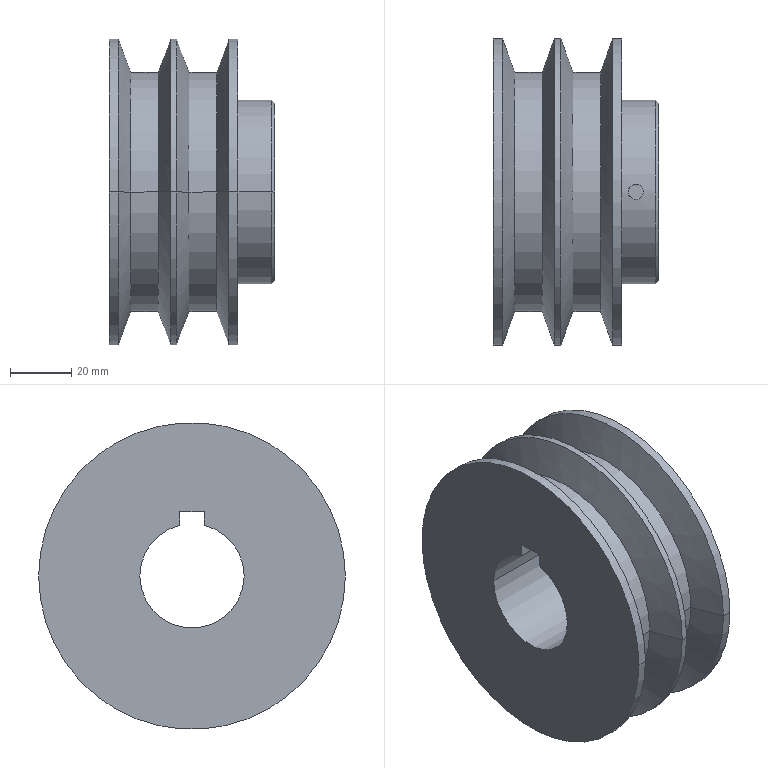Part | SolidWorks | features ICE 2, Chamfer 1, HoleWzd 1, Revolution 1 | 1 solid | 33 faces | box 54 x 100 x 100 mm | volume 231745 mm3 | cylinder 17 | cone 10 | plane 6 | commonest cylinder face diameters 100 x6 78 x4 34 x3 5 x2 60 x2
STEP:
#1=CARTESIAN_POINT('',(54.,29.,0.));
#2=VERTEX_POINT('',#1);
#3=CARTESIAN_POINT('',(54.,-29.,0.));
#4=VERTEX_POINT('',#3);
#5=CARTESIAN_POINT('',(54.,0.,0.));
#6=DIRECTION('',(1.,0.,0.));
#7=DIRECTION('',(0.,1.,0.));
#8=AXIS2_PLACEMENT_3D('',#5,#6,#7);
#9=CIRCLE('',#8,29.);
#10=EDGE_CURVE('',#2,#4,#9,.T.);
#11=ORIENTED_EDGE('',*,*,#10,.F.);
#12=CARTESIAN_POINT('',(53.,30.,0.));
#13=VERTEX_POINT('',#12);
#14=CARTESIAN_POINT('',(54.,29.,0.));
#15=DIRECTION('',(-0.7071,0.7071,0.));
#16=VECTOR('',#15,1000.);
#17=LINE('',#14,#16);
#18=EDGE_CURVE('',#2,#13,#17,.T.);
#19=ORIENTED_EDGE('',*,*,#18,.T.);
#20=CARTESIAN_POINT('',(53.,-30.,0.));
#21=VERTEX_POINT('',#20);
#22=CARTESIAN_POINT('',(53.,0.,0.));
#23=DIRECTION('',(-1.,0.,0.));
#24=DIRECTION('',(0.,1.,0.));
#25=AXIS2_PLACEMENT_3D('',#22,#23,#24);
#26=CIRCLE('',#25,30.);
#27=EDGE_CURVE('',#21,#13,#26,.T.);
#28=ORIENTED_EDGE('',*,*,#27,.F.);
#29=CARTESIAN_POINT('',(54.,-29.,0.));
#30=DIRECTION('',(-0.7071,-0.7071,0.));
#31=VECTOR('',#30,1000.);
#32=LINE('',#29,#31);
#33=EDGE_CURVE('',#4,#21,#32,.T.);
#34=ORIENTED_EDGE('',*,*,#33,.F.);
#35=EDGE_LOOP('',(#11,#19,#28,#34));
#36=FACE_OUTER_BOUND('',#35,.T.);
#37=CARTESIAN_POINT('',(54.,0.,0.));
#38=DIRECTION('',(-1.,0.,0.));
#39=DIRECTION('',(0.,-1.,0.));
#40=AXIS2_PLACEMENT_3D('',#37,#38,#39);
#41=CONICAL_SURFACE('',#40,29.,0.7854);
#42=ADVANCED_FACE('',(#36),#41,.T.);
#43=CARTESIAN_POINT('',(44.,0.,30.));
#44=VERTEX_POINT('',#43);
#45=CARTESIAN_POINT('',(49.,0.,30.));
#46=VERTEX_POINT('',#45);
#47=CARTESIAN_POINT('',(44.,0.,30.));
#48=CARTESIAN_POINT('',(44.,-0.1653,30.));
#49=CARTESIAN_POINT('',(44.016,-0.3277,29.999));
#50=CARTESIAN_POINT('',(44.08,-0.6474,29.993));
#51=CARTESIAN_POINT('',(44.128,-0.8062,29.99));
#52=CARTESIAN_POINT('',(44.253,-1.109,29.98));
#53=CARTESIAN_POINT('',(44.33,-1.253,29.974));
#54=CARTESIAN_POINT('',(44.512,-1.524,29.962));
#55=CARTESIAN_POINT('',(44.617,-1.653,29.955));
#56=CARTESIAN_POINT('',(44.848,-1.883,29.941));
#57=CARTESIAN_POINT('',(44.974,-1.987,29.934));
#58=CARTESIAN_POINT('',(45.247,-2.17,29.922));
#59=CARTESIAN_POINT('',(45.392,-2.247,29.916));
#60=CARTESIAN_POINT('',(45.693,-2.372,29.906));
#61=CARTESIAN_POINT('',(45.851,-2.42,29.902));
#62=CARTESIAN_POINT('',(46.174,-2.484,29.897));
#63=CARTESIAN_POINT('',(46.336,-2.5,29.896));
#64=CARTESIAN_POINT('',(46.662,-2.5,29.896));
#65=CARTESIAN_POINT('',(46.828,-2.484,29.897));
#66=CARTESIAN_POINT('',(47.149,-2.42,29.902));
#67=CARTESIAN_POINT('',(47.305,-2.373,29.906));
#68=CARTESIAN_POINT('',(47.607,-2.247,29.916));
#69=CARTESIAN_POINT('',(47.754,-2.169,29.922));
#70=CARTESIAN_POINT('',(48.024,-1.988,29.934));
#71=CARTESIAN_POINT('',(48.151,-1.885,29.941));
#72=CARTESIAN_POINT('',(48.384,-1.651,29.955));
#73=CARTESIAN_POINT('',(48.488,-1.525,29.962));
#74=CARTESIAN_POINT('',(48.669,-1.254,29.974));
#75=CARTESIAN_POINT('',(48.747,-1.108,29.98));
#76=CARTESIAN_POINT('',(48.872,-0.8053,29.99));
#77=CARTESIAN_POINT('',(48.92,-0.6495,29.993));
#78=CARTESIAN_POINT('',(48.984,-0.329,29.999));
#79=CARTESIAN_POINT('',(49.,-0.1632,30.));
#80=CARTESIAN_POINT('',(49.,0.,30.));
#81=B_SPLINE_CURVE_WITH_KNOTS('',3,(#47,#48,#49,#50,#51,#52,#53,#54,#55,#56,#57,#58,#59,#60,#61,#62,#63,#64,#65,#66,#67,#68,#69,#70,#71,#72,#73,#74,#75,#76,#77,#78,#79,#80),.UNSPECIFIED.,.F.,.F.,(4,2,2,2,2,2,2,2,2,2,2,2,2,2,2,2,4),(0.,0.0004887,0.0009774,0.001466,0.001955,0.002444,0.002932,0.003421,0.00391,0.004398,0.004887,0.005376,0.005865,0.006353,0.006842,0.007331,0.00782),.UNSPECIFIED.);
#82=EDGE_CURVE('',#44,#46,#81,.T.);
#83=ORIENTED_EDGE('',*,*,#82,.T.);
#84=CARTESIAN_POINT('',(49.,0.,21.));
#85=VERTEX_POINT('',#84);
#86=CARTESIAN_POINT('',(49.,0.,0.));
#87=DIRECTION('',(0.,0.,-1.));
#88=VECTOR('',#87,1000.);
#89=LINE('',#86,#88);
#90=EDGE_CURVE('',#46,#85,#89,.T.);
#91=ORIENTED_EDGE('',*,*,#90,.T.);
#92=CARTESIAN_POINT('',(44.,0.,21.));
#93=VERTEX_POINT('',#92);
#94=CARTESIAN_POINT('',(46.5,0.,21.));
#95=DIRECTION('',(0.,0.,-1.));
#96=DIRECTION('',(1.,0.,0.));
#97=AXIS2_PLACEMENT_3D('',#94,#95,#96);
#98=CIRCLE('',#97,2.5);
#99=EDGE_CURVE('',#85,#93,#98,.T.);
#100=ORIENTED_EDGE('',*,*,#99,.T.);
#101=CARTESIAN_POINT('',(44.,0.,0.));
#102=DIRECTION('',(0.,0.,-1.));
#103=VECTOR('',#102,1000.);
#104=LINE('',#101,#103);
#105=EDGE_CURVE('',#44,#93,#104,.T.);
#106=ORIENTED_EDGE('',*,*,#105,.F.);
#107=EDGE_LOOP('',(#83,#91,#100,#106));
#108=FACE_OUTER_BOUND('',#107,.T.);
#109=CARTESIAN_POINT('',(46.5,0.,0.));
#110=DIRECTION('',(0.,0.,-1.));
#111=DIRECTION('',(-1.,0.,0.));
#112=AXIS2_PLACEMENT_3D('',#109,#110,#111);
#113=CYLINDRICAL_SURFACE('',#112,2.5);
#114=ADVANCED_FACE('',(#108),#113,.F.);
#115=CARTESIAN_POINT('',(0.,17.,0.));
#116=VERTEX_POINT('',#115);
#117=CARTESIAN_POINT('',(0.,-17.,0.));
#118=VERTEX_POINT('',#117);
#119=CARTESIAN_POINT('',(0.,0.,0.));
#120=DIRECTION('',(-1.,0.,0.));
#121=DIRECTION('',(0.,-1.,0.));
#122=AXIS2_PLACEMENT_3D('',#119,#120,#121);
#123=CIRCLE('',#122,17.);
#124=EDGE_CURVE('',#116,#118,#123,.T.);
#125=ORIENTED_EDGE('',*,*,#124,.T.);
#126=CARTESIAN_POINT('',(54.,-17.,0.));
#127=VERTEX_POINT('',#126);
#128=CARTESIAN_POINT('',(-16.,-17.,0.));
#129=DIRECTION('',(1.,0.,0.));
#130=VECTOR('',#129,1000.);
#131=LINE('',#128,#130);
#132=EDGE_CURVE('',#118,#127,#131,.T.);
#133=ORIENTED_EDGE('',*,*,#132,.T.);
#134=CARTESIAN_POINT('',(54.,17.,0.));
#135=VERTEX_POINT('',#134);
#136=CARTESIAN_POINT('',(54.,0.,0.));
#137=DIRECTION('',(1.,0.,0.));
#138=DIRECTION('',(0.,1.,0.));
#139=AXIS2_PLACEMENT_3D('',#136,#137,#138);
#140=CIRCLE('',#139,17.);
#141=EDGE_CURVE('',#127,#135,#140,.T.);
#142=ORIENTED_EDGE('',*,*,#141,.T.);
#143=CARTESIAN_POINT('',(-16.,17.,0.));
#144=DIRECTION('',(1.,0.,0.));
#145=VECTOR('',#144,1000.);
#146=LINE('',#143,#145);
#147=EDGE_CURVE('',#116,#135,#146,.T.);
#148=ORIENTED_EDGE('',*,*,#147,.F.);
#149=EDGE_LOOP('',(#125,#133,#142,#148));
#150=FACE_OUTER_BOUND('',#149,.T.);
#151=CARTESIAN_POINT('',(-16.,0.,0.));
#152=DIRECTION('',(1.,0.,0.));
#153=DIRECTION('',(0.,1.,0.));
#154=AXIS2_PLACEMENT_3D('',#151,#152,#153);
#155=CYLINDRICAL_SURFACE('',#154,17.);
#156=ADVANCED_FACE('',(#150),#155,.F.);
#157=CARTESIAN_POINT('',(0.,4.,16.523));
#158=VERTEX_POINT('',#157);
#159=CARTESIAN_POINT('',(0.,0.,0.));
#160=DIRECTION('',(-1.,0.,0.));
#161=DIRECTION('',(0.,-1.,0.));
#162=AXIS2_PLACEMENT_3D('',#159,#160,#161);
#163=CIRCLE('',#162,17.);
#164=EDGE_CURVE('',#158,#116,#163,.T.);
#165=ORIENTED_EDGE('',*,*,#164,.T.);
#166=ORIENTED_EDGE('',*,*,#147,.T.);
#167=CARTESIAN_POINT('',(54.,4.,16.523));
#168=VERTEX_POINT('',#167);
#169=CARTESIAN_POINT('',(54.,0.,0.));
#170=DIRECTION('',(1.,0.,0.));
#171=DIRECTION('',(0.,1.,0.));
#172=AXIS2_PLACEMENT_3D('',#169,#170,#171);
#173=CIRCLE('',#172,17.);
#174=EDGE_CURVE('',#135,#168,#173,.T.);
#175=ORIENTED_EDGE('',*,*,#174,.T.);
#176=CARTESIAN_POINT('',(-16.,4.,16.523));
#177=DIRECTION('',(-1.,0.,0.));
#178=VECTOR('',#177,1000.);
#179=LINE('',#176,#178);
#180=EDGE_CURVE('',#168,#158,#179,.T.);
#181=ORIENTED_EDGE('',*,*,#180,.T.);
#182=EDGE_LOOP('',(#165,#166,#175,#181));
#183=FACE_OUTER_BOUND('',#182,.T.);
#184=CARTESIAN_POINT('',(-16.,0.,0.));
#185=DIRECTION('',(1.,0.,0.));
#186=DIRECTION('',(0.,1.,0.));
#187=AXIS2_PLACEMENT_3D('',#184,#185,#186);
#188=CYLINDRICAL_SURFACE('',#187,17.);
#189=ADVANCED_FACE('',(#183),#188,.F.);
#190=ORIENTED_EDGE('',*,*,#82,.F.);
#191=CARTESIAN_POINT('',(49.,0.,30.));
#192=CARTESIAN_POINT('',(49.,0.1632,30.));
#193=CARTESIAN_POINT('',(48.984,0.3254,29.999));
#194=CARTESIAN_POINT('',(48.92,0.6478,29.993));
#195=CARTESIAN_POINT('',(48.872,0.8057,29.99));
#196=CARTESIAN_POINT('',(48.748,1.107,29.98));
#197=CARTESIAN_POINT('',(48.67,1.252,29.974));
#198=CARTESIAN_POINT('',(48.488,1.525,29.962));
#199=CARTESIAN_POINT('',(48.384,1.651,29.955));
#200=CARTESIAN_POINT('',(48.154,1.882,29.941));
#201=CARTESIAN_POINT('',(48.025,1.987,29.934));
#202=CARTESIAN_POINT('',(47.754,2.169,29.922));
#203=CARTESIAN_POINT('',(47.61,2.246,29.916));
#204=CARTESIAN_POINT('',(47.308,2.372,29.906));
#205=CARTESIAN_POINT('',(47.149,2.42,29.902));
#206=CARTESIAN_POINT('',(46.829,2.484,29.897));
#207=CARTESIAN_POINT('',(46.667,2.5,29.896));
#208=CARTESIAN_POINT('',(46.337,2.5,29.896));
#209=CARTESIAN_POINT('',(46.174,2.484,29.897));
#210=CARTESIAN_POINT('',(45.854,2.421,29.902));
#211=CARTESIAN_POINT('',(45.696,2.373,29.906));
#212=CARTESIAN_POINT('',(45.393,2.247,29.916));
#213=CARTESIAN_POINT('',(45.249,2.171,29.921));
#214=CARTESIAN_POINT('',(44.978,1.99,29.934));
#215=CARTESIAN_POINT('',(44.849,1.884,29.941));
#216=CARTESIAN_POINT('',(44.618,1.654,29.955));
#217=CARTESIAN_POINT('',(44.515,1.528,29.961));
#218=CARTESIAN_POINT('',(44.332,1.255,29.974));
#219=CARTESIAN_POINT('',(44.254,1.11,29.98));
#220=CARTESIAN_POINT('',(44.066,0.6587,29.994));
#221=CARTESIAN_POINT('',(44.,0.3304,30.));
#222=CARTESIAN_POINT('',(44.,0.,30.));
#223=B_SPLINE_CURVE_WITH_KNOTS('',3,(#191,#192,#193,#194,#195,#196,#197,#198,#199,#200,#201,#202,#203,#204,#205,#206,#207,#208,#209,#210,#211,#212,#213,#214,#215,#216,#217,#218,#219,#220,#221,#222),.UNSPECIFIED.,.F.,.F.,(4,2,2,2,2,2,2,2,2,2,2,2,2,2,2,4),(0.00782,0.008308,0.008797,0.009285,0.009774,0.01026,0.01075,0.01124,0.01173,0.01222,0.01271,0.01319,0.01368,0.01417,0.01466,0.01564),.UNSPECIFIED.);
#224=EDGE_CURVE('',#46,#44,#223,.T.);
#225=ORIENTED_EDGE('',*,*,#224,.F.);
#226=EDGE_LOOP('',(#190,#225));
#227=FACE_BOUND('',#226,.T.);
#228=CARTESIAN_POINT('',(42.,30.,0.));
#229=VERTEX_POINT('',#228);
#230=CARTESIAN_POINT('',(42.,-30.,0.));
#231=VERTEX_POINT('',#230);
#232=CARTESIAN_POINT('',(42.,0.,0.));
#233=DIRECTION('',(1.,0.,0.));
#234=DIRECTION('',(0.,1.,0.));
#235=AXIS2_PLACEMENT_3D('',#232,#233,#234);
#236=CIRCLE('',#235,30.);
#237=EDGE_CURVE('',#229,#231,#236,.T.);
#238=ORIENTED_EDGE('',*,*,#237,.T.);
#239=CARTESIAN_POINT('',(54.,-30.,0.));
#240=DIRECTION('',(1.,0.,0.));
#241=VECTOR('',#240,1000.);
#242=LINE('',#239,#241);
#243=EDGE_CURVE('',#231,#21,#242,.T.);
#244=ORIENTED_EDGE('',*,*,#243,.T.);
#245=ORIENTED_EDGE('',*,*,#27,.T.);
#246=CARTESIAN_POINT('',(54.,30.,0.));
#247=DIRECTION('',(1.,0.,0.));
#248=VECTOR('',#247,1000.);
#249=LINE('',#246,#248);
#250=EDGE_CURVE('',#229,#13,#249,.T.);
#251=ORIENTED_EDGE('',*,*,#250,.F.);
#252=EDGE_LOOP('',(#238,#244,#245,#251));
#253=FACE_OUTER_BOUND('',#252,.T.);
#254=CARTESIAN_POINT('',(54.,0.,0.));
#255=DIRECTION('',(1.,0.,0.));
#256=DIRECTION('',(0.,1.,0.));
#257=AXIS2_PLACEMENT_3D('',#254,#255,#256);
#258=CYLINDRICAL_SURFACE('',#257,30.);
#259=ADVANCED_FACE('',(#227,#253),#258,.T.);
#260=CARTESIAN_POINT('',(39.,50.,0.));
#261=VERTEX_POINT('',#260);
#262=CARTESIAN_POINT('',(39.,-50.,0.));
#263=VERTEX_POINT('',#262);
#264=CARTESIAN_POINT('',(39.,0.,0.));
#265=DIRECTION('',(1.,0.,0.));
#266=DIRECTION('',(0.,1.,0.));
#267=AXIS2_PLACEMENT_3D('',#264,#265,#266);
#268=CIRCLE('',#267,50.);
#269=EDGE_CURVE('',#261,#263,#268,.T.);
#270=ORIENTED_EDGE('',*,*,#269,.T.);
#271=CARTESIAN_POINT('',(42.,-50.,0.));
#272=VERTEX_POINT('',#271);
#273=CARTESIAN_POINT('',(54.,-50.,0.));
#274=DIRECTION('',(1.,0.,0.));
#275=VECTOR('',#274,1000.);
#276=LINE('',#273,#275);
#277=EDGE_CURVE('',#263,#272,#276,.T.);
#278=ORIENTED_EDGE('',*,*,#277,.T.);
#279=CARTESIAN_POINT('',(42.,50.,0.));
#280=VERTEX_POINT('',#279);
#281=CARTESIAN_POINT('',(42.,0.,0.));
#282=DIRECTION('',(1.,0.,0.));
#283=DIRECTION('',(0.,1.,0.));
#284=AXIS2_PLACEMENT_3D('',#281,#282,#283);
#285=CIRCLE('',#284,50.);
#286=EDGE_CURVE('',#280,#272,#285,.T.);
#287=ORIENTED_EDGE('',*,*,#286,.F.);
#288=CARTESIAN_POINT('',(54.,50.,0.));
#289=DIRECTION('',(1.,0.,0.));
#290=VECTOR('',#289,1000.);
#291=LINE('',#288,#290);
#292=EDGE_CURVE('',#261,#280,#291,.T.);
#293=ORIENTED_EDGE('',*,*,#292,.F.);
#294=EDGE_LOOP('',(#270,#278,#287,#293));
#295=FACE_OUTER_BOUND('',#294,.T.);
#296=CARTESIAN_POINT('',(54.,0.,0.));
#297=DIRECTION('',(1.,0.,0.));
#298=DIRECTION('',(0.,1.,0.));
#299=AXIS2_PLACEMENT_3D('',#296,#297,#298);
#300=CYLINDRICAL_SURFACE('',#299,50.);
#301=ADVANCED_FACE('',(#295),#300,.T.);
#302=CARTESIAN_POINT('',(34.996,39.,0.));
#303=VERTEX_POINT('',#302);
#304=CARTESIAN_POINT('',(34.996,-39.,0.));
#305=VERTEX_POINT('',#304);
#306=CARTESIAN_POINT('',(34.996,0.,0.));
#307=DIRECTION('',(1.,0.,0.));
#308=DIRECTION('',(0.,1.,0.));
#309=AXIS2_PLACEMENT_3D('',#306,#307,#308);
#310=CIRCLE('',#309,39.);
#311=EDGE_CURVE('',#303,#305,#310,.T.);
#312=ORIENTED_EDGE('',*,*,#311,.T.);
#313=CARTESIAN_POINT('',(39.,-50.,0.));
#314=DIRECTION('',(0.342,-0.9397,0.));
#315=VECTOR('',#314,1000.);
#316=LINE('',#313,#315);
#317=EDGE_CURVE('',#305,#263,#316,.T.);
#318=ORIENTED_EDGE('',*,*,#317,.T.);
#319=ORIENTED_EDGE('',*,*,#269,.F.);
#320=CARTESIAN_POINT('',(39.,50.,0.));
#321=DIRECTION('',(0.342,0.9397,0.));
#322=VECTOR('',#321,1000.);
#323=LINE('',#320,#322);
#324=EDGE_CURVE('',#303,#261,#323,.T.);
#325=ORIENTED_EDGE('',*,*,#324,.F.);
#326=EDGE_LOOP('',(#312,#318,#319,#325));
#327=FACE_OUTER_BOUND('',#326,.T.);
#328=CARTESIAN_POINT('',(39.,0.,0.));
#329=DIRECTION('',(1.,0.,0.));
#330=DIRECTION('',(0.,1.,0.));
#331=AXIS2_PLACEMENT_3D('',#328,#329,#330);
#332=CONICAL_SURFACE('',#331,50.,1.222);
#333=ADVANCED_FACE('',(#327),#332,.T.);
#334=CARTESIAN_POINT('',(26.004,39.,0.));
#335=VERTEX_POINT('',#334);
#336=CARTESIAN_POINT('',(26.004,-39.,0.));
#337=VERTEX_POINT('',#336);
#338=CARTESIAN_POINT('',(26.004,0.,0.));
#339=DIRECTION('',(1.,0.,0.));
#340=DIRECTION('',(0.,1.,0.));
#341=AXIS2_PLACEMENT_3D('',#338,#339,#340);
#342=CIRCLE('',#341,39.);
#343=EDGE_CURVE('',#335,#337,#342,.T.);
#344=ORIENTED_EDGE('',*,*,#343,.T.);
#345=CARTESIAN_POINT('',(54.,-39.,0.));
#346=DIRECTION('',(1.,0.,0.));
#347=VECTOR('',#346,1000.);
#348=LINE('',#345,#347);
#349=EDGE_CURVE('',#337,#305,#348,.T.);
#350=ORIENTED_EDGE('',*,*,#349,.T.);
#351=ORIENTED_EDGE('',*,*,#311,.F.);
#352=CARTESIAN_POINT('',(54.,39.,0.));
#353=DIRECTION('',(1.,0.,0.));
#354=VECTOR('',#353,1000.);
#355=LINE('',#352,#354);
#356=EDGE_CURVE('',#335,#303,#355,.T.);
#357=ORIENTED_EDGE('',*,*,#356,.F.);
#358=EDGE_LOOP('',(#344,#350,#351,#357));
#359=FACE_OUTER_BOUND('',#358,.T.);
#360=CARTESIAN_POINT('',(54.,0.,0.));
#361=DIRECTION('',(1.,0.,0.));
#362=DIRECTION('',(0.,1.,0.));
#363=AXIS2_PLACEMENT_3D('',#360,#361,#362);
#364=CYLINDRICAL_SURFACE('',#363,39.);
#365=ADVANCED_FACE('',(#359),#364,.T.);
#366=ORIENTED_EDGE('',*,*,#343,.F.);
#367=CARTESIAN_POINT('',(22.,50.,0.));
#368=VERTEX_POINT('',#367);
#369=CARTESIAN_POINT('',(26.004,39.,0.));
#370=DIRECTION('',(-0.342,0.9397,0.));
#371=VECTOR('',#370,1000.);
#372=LINE('',#369,#371);
#373=EDGE_CURVE('',#335,#368,#372,.T.);
#374=ORIENTED_EDGE('',*,*,#373,.T.);
#375=CARTESIAN_POINT('',(22.,-50.,0.));
#376=VERTEX_POINT('',#375);
#377=CARTESIAN_POINT('',(22.,0.,0.));
#378=DIRECTION('',(1.,0.,0.));
#379=DIRECTION('',(0.,1.,0.));
#380=AXIS2_PLACEMENT_3D('',#377,#378,#379);
#381=CIRCLE('',#380,50.);
#382=EDGE_CURVE('',#368,#376,#381,.T.);
#383=ORIENTED_EDGE('',*,*,#382,.T.);
#384=CARTESIAN_POINT('',(26.004,-39.,0.));
#385=DIRECTION('',(-0.342,-0.9397,0.));
#386=VECTOR('',#385,1000.);
#387=LINE('',#384,#386);
#388=EDGE_CURVE('',#337,#376,#387,.T.);
#389=ORIENTED_EDGE('',*,*,#388,.F.);
#390=EDGE_LOOP('',(#366,#374,#383,#389));
#391=FACE_OUTER_BOUND('',#390,.T.);
#392=CARTESIAN_POINT('',(26.004,0.,0.));
#393=DIRECTION('',(-1.,0.,0.));
#394=DIRECTION('',(0.,-1.,0.));
#395=AXIS2_PLACEMENT_3D('',#392,#393,#394);
#396=CONICAL_SURFACE('',#395,39.,1.222);
#397=ADVANCED_FACE('',(#391),#396,.T.);
#398=CARTESIAN_POINT('',(20.,50.,0.));
#399=VERTEX_POINT('',#398);
#400=CARTESIAN_POINT('',(20.,-50.,0.));
#401=VERTEX_POINT('',#400);
#402=CARTESIAN_POINT('',(20.,0.,0.));
#403=DIRECTION('',(1.,0.,0.));
#404=DIRECTION('',(0.,1.,0.));
#405=AXIS2_PLACEMENT_3D('',#402,#403,#404);
#406=CIRCLE('',#405,50.);
#407=EDGE_CURVE('',#399,#401,#406,.T.);
#408=ORIENTED_EDGE('',*,*,#407,.T.);
#409=CARTESIAN_POINT('',(54.,-50.,0.));
#410=DIRECTION('',(1.,0.,0.));
#411=VECTOR('',#410,1000.);
#412=LINE('',#409,#411);
#413=EDGE_CURVE('',#401,#376,#412,.T.);
#414=ORIENTED_EDGE('',*,*,#413,.T.);
#415=ORIENTED_EDGE('',*,*,#382,.F.);
#416=CARTESIAN_POINT('',(54.,50.,0.));
#417=DIRECTION('',(1.,0.,0.));
#418=VECTOR('',#417,1000.);
#419=LINE('',#416,#418);
#420=EDGE_CURVE('',#399,#368,#419,.T.);
#421=ORIENTED_EDGE('',*,*,#420,.F.);
#422=EDGE_LOOP('',(#408,#414,#415,#421));
#423=FACE_OUTER_BOUND('',#422,.T.);
#424=CARTESIAN_POINT('',(54.,0.,0.));
#425=DIRECTION('',(1.,0.,0.));
#426=DIRECTION('',(0.,1.,0.));
#427=AXIS2_PLACEMENT_3D('',#424,#425,#426);
#428=CYLINDRICAL_SURFACE('',#427,50.);
#429=ADVANCED_FACE('',(#423),#428,.T.);
#430=CARTESIAN_POINT('',(15.996,39.,0.));
#431=VERTEX_POINT('',#430);
#432=CARTESIAN_POINT('',(15.996,-39.,0.));
#433=VERTEX_POINT('',#432);
#434=CARTESIAN_POINT('',(15.996,0.,0.));
#435=DIRECTION('',(1.,0.,0.));
#436=DIRECTION('',(0.,1.,0.));
#437=AXIS2_PLACEMENT_3D('',#434,#435,#436);
#438=CIRCLE('',#437,39.);
#439=EDGE_CURVE('',#431,#433,#438,.T.);
#440=ORIENTED_EDGE('',*,*,#439,.T.);
#441=CARTESIAN_POINT('',(20.,-50.,0.));
#442=DIRECTION('',(0.342,-0.9397,0.));
#443=VECTOR('',#442,1000.);
#444=LINE('',#441,#443);
#445=EDGE_CURVE('',#433,#401,#444,.T.);
#446=ORIENTED_EDGE('',*,*,#445,.T.);
#447=ORIENTED_EDGE('',*,*,#407,.F.);
#448=CARTESIAN_POINT('',(20.,50.,0.));
#449=DIRECTION('',(0.342,0.9397,0.));
#450=VECTOR('',#449,1000.);
#451=LINE('',#448,#450);
#452=EDGE_CURVE('',#431,#399,#451,.T.);
#453=ORIENTED_EDGE('',*,*,#452,.F.);
#454=EDGE_LOOP('',(#440,#446,#447,#453));
#455=FACE_OUTER_BOUND('',#454,.T.);
#456=CARTESIAN_POINT('',(20.,0.,0.));
#457=DIRECTION('',(1.,0.,0.));
#458=DIRECTION('',(0.,1.,0.));
#459=AXIS2_PLACEMENT_3D('',#456,#457,#458);
#460=CONICAL_SURFACE('',#459,50.,1.222);
#461=ADVANCED_FACE('',(#455),#460,.T.);
#462=CARTESIAN_POINT('',(7.004,39.,0.));
#463=VERTEX_POINT('',#462);
#464=CARTESIAN_POINT('',(7.004,-39.,0.));
#465=VERTEX_POINT('',#464);
#466=CARTESIAN_POINT('',(7.004,0.,0.));
#467=DIRECTION('',(1.,0.,0.));
#468=DIRECTION('',(0.,1.,0.));
#469=AXIS2_PLACEMENT_3D('',#466,#467,#468);
#470=CIRCLE('',#469,39.);
#471=EDGE_CURVE('',#463,#465,#470,.T.);
#472=ORIENTED_EDGE('',*,*,#471,.T.);
#473=CARTESIAN_POINT('',(54.,-39.,0.));
#474=DIRECTION('',(1.,0.,0.));
#475=VECTOR('',#474,1000.);
#476=LINE('',#473,#475);
#477=EDGE_CURVE('',#465,#433,#476,.T.);
#478=ORIENTED_EDGE('',*,*,#477,.T.);
#479=ORIENTED_EDGE('',*,*,#439,.F.);
#480=CARTESIAN_POINT('',(54.,39.,0.));
#481=DIRECTION('',(1.,0.,0.));
#482=VECTOR('',#481,1000.);
#483=LINE('',#480,#482);
#484=EDGE_CURVE('',#463,#431,#483,.T.);
#485=ORIENTED_EDGE('',*,*,#484,.F.);
#486=EDGE_LOOP('',(#472,#478,#479,#485));
#487=FACE_OUTER_BOUND('',#486,.T.);
#488=CARTESIAN_POINT('',(54.,0.,0.));
#489=DIRECTION('',(1.,0.,0.));
#490=DIRECTION('',(0.,1.,0.));
#491=AXIS2_PLACEMENT_3D('',#488,#489,#490);
#492=CYLINDRICAL_SURFACE('',#491,39.);
#493=ADVANCED_FACE('',(#487),#492,.T.);
#494=ORIENTED_EDGE('',*,*,#471,.F.);
#495=CARTESIAN_POINT('',(3.,50.,0.));
#496=VERTEX_POINT('',#495);
#497=CARTESIAN_POINT('',(7.004,39.,0.));
#498=DIRECTION('',(-0.342,0.9397,0.));
#499=VECTOR('',#498,1000.);
#500=LINE('',#497,#499);
#501=EDGE_CURVE('',#463,#496,#500,.T.);
#502=ORIENTED_EDGE('',*,*,#501,.T.);
#503=CARTESIAN_POINT('',(3.,-50.,0.));
#504=VERTEX_POINT('',#503);
#505=CARTESIAN_POINT('',(3.,0.,0.));
#506=DIRECTION('',(1.,0.,0.));
#507=DIRECTION('',(0.,1.,0.));
#508=AXIS2_PLACEMENT_3D('',#505,#506,#507);
#509=CIRCLE('',#508,50.);
#510=EDGE_CURVE('',#496,#504,#509,.T.);
#511=ORIENTED_EDGE('',*,*,#510,.T.);
#512=CARTESIAN_POINT('',(7.004,-39.,0.));
#513=DIRECTION('',(-0.342,-0.9397,0.));
#514=VECTOR('',#513,1000.);
#515=LINE('',#512,#514);
#516=EDGE_CURVE('',#465,#504,#515,.T.);
#517=ORIENTED_EDGE('',*,*,#516,.F.);
#518=EDGE_LOOP('',(#494,#502,#511,#517));
#519=FACE_OUTER_BOUND('',#518,.T.);
#520=CARTESIAN_POINT('',(7.004,0.,0.));
#521=DIRECTION('',(-1.,0.,0.));
#522=DIRECTION('',(0.,-1.,0.));
#523=AXIS2_PLACEMENT_3D('',#520,#521,#522);
#524=CONICAL_SURFACE('',#523,39.,1.222);
#525=ADVANCED_FACE('',(#519),#524,.T.);
#526=CARTESIAN_POINT('',(0.,50.,0.));
#527=VERTEX_POINT('',#526);
#528=CARTESIAN_POINT('',(0.,-50.,0.));
#529=VERTEX_POINT('',#528);
#530=CARTESIAN_POINT('',(0.,0.,0.));
#531=DIRECTION('',(1.,0.,0.));
#532=DIRECTION('',(0.,1.,0.));
#533=AXIS2_PLACEMENT_3D('',#530,#531,#532);
#534=CIRCLE('',#533,50.);
#535=EDGE_CURVE('',#527,#529,#534,.T.);
#536=ORIENTED_EDGE('',*,*,#535,.T.);
#537=CARTESIAN_POINT('',(54.,-50.,0.));
#538=DIRECTION('',(1.,0.,0.));
#539=VECTOR('',#538,1000.);
#540=LINE('',#537,#539);
#541=EDGE_CURVE('',#529,#504,#540,.T.);
#542=ORIENTED_EDGE('',*,*,#541,.T.);
#543=ORIENTED_EDGE('',*,*,#510,.F.);
#544=CARTESIAN_POINT('',(54.,50.,0.));
#545=DIRECTION('',(1.,0.,0.));
#546=VECTOR('',#545,1000.);
#547=LINE('',#544,#546);
#548=EDGE_CURVE('',#527,#496,#547,.T.);
#549=ORIENTED_EDGE('',*,*,#548,.F.);
#550=EDGE_LOOP('',(#536,#542,#543,#549));
#551=FACE_OUTER_BOUND('',#550,.T.);
#552=CARTESIAN_POINT('',(54.,0.,0.));
#553=DIRECTION('',(1.,0.,0.));
#554=DIRECTION('',(0.,1.,0.));
#555=AXIS2_PLACEMENT_3D('',#552,#553,#554);
#556=CYLINDRICAL_SURFACE('',#555,50.);
#557=ADVANCED_FACE('',(#551),#556,.T.);
#558=CARTESIAN_POINT('',(0.,-4.,16.523));
#559=VERTEX_POINT('',#558);
#560=CARTESIAN_POINT('',(0.,-4.,21.));
#561=VERTEX_POINT('',#560);
#562=CARTESIAN_POINT('',(0.,-4.,0.));
#563=DIRECTION('',(0.,0.,1.));
#564=VECTOR('',#563,1000.);
#565=LINE('',#562,#564);
#566=EDGE_CURVE('',#559,#561,#565,.T.);
#567=ORIENTED_EDGE('',*,*,#566,.F.);
#568=CARTESIAN_POINT('',(0.,0.,0.));
#569=DIRECTION('',(-1.,0.,0.));
#570=DIRECTION('',(0.,-1.,0.));
#571=AXIS2_PLACEMENT_3D('',#568,#569,#570);
#572=CIRCLE('',#571,17.);
#573=EDGE_CURVE('',#118,#559,#572,.T.);
#574=ORIENTED_EDGE('',*,*,#573,.F.);
#575=ORIENTED_EDGE('',*,*,#124,.F.);
#576=ORIENTED_EDGE('',*,*,#164,.F.);
#577=CARTESIAN_POINT('',(0.,4.,21.));
#578=VERTEX_POINT('',#577);
#579=CARTESIAN_POINT('',(0.,4.,0.));
#580=DIRECTION('',(0.,0.,-1.));
#581=VECTOR('',#580,1000.);
#582=LINE('',#579,#581);
#583=EDGE_CURVE('',#578,#158,#582,.T.);
#584=ORIENTED_EDGE('',*,*,#583,.F.);
#585=CARTESIAN_POINT('',(0.,0.,21.));
#586=DIRECTION('',(0.,1.,0.));
#587=VECTOR('',#586,1000.);
#588=LINE('',#585,#587);
#589=EDGE_CURVE('',#561,#578,#588,.T.);
#590=ORIENTED_EDGE('',*,*,#589,.F.);
#591=EDGE_LOOP('',(#567,#574,#575,#576,#584,#590));
#592=FACE_BOUND('',#591,.T.);
#593=ORIENTED_EDGE('',*,*,#535,.F.);
#594=CARTESIAN_POINT('',(0.,0.,0.));
#595=DIRECTION('',(1.,0.,0.));
#596=DIRECTION('',(0.,1.,0.));
#597=AXIS2_PLACEMENT_3D('',#594,#595,#596);
#598=CIRCLE('',#597,50.);
#599=EDGE_CURVE('',#529,#527,#598,.T.);
#600=ORIENTED_EDGE('',*,*,#599,.F.);
#601=EDGE_LOOP('',(#593,#600));
#602=FACE_OUTER_BOUND('',#601,.T.);
#603=CARTESIAN_POINT('',(0.,0.,0.));
#604=DIRECTION('',(-1.,0.,0.));
#605=DIRECTION('',(0.,-1.,0.));
#606=AXIS2_PLACEMENT_3D('',#603,#604,#605);
#607=PLANE('',#606);
#608=ADVANCED_FACE('',(#592,#602),#607,.T.);
#609=ORIENTED_EDGE('',*,*,#541,.F.);
#610=ORIENTED_EDGE('',*,*,#599,.T.);
#611=ORIENTED_EDGE('',*,*,#548,.T.);
#612=CARTESIAN_POINT('',(3.,0.,0.));
#613=DIRECTION('',(1.,0.,0.));
#614=DIRECTION('',(0.,1.,0.));
#615=AXIS2_PLACEMENT_3D('',#612,#613,#614);
#616=CIRCLE('',#615,50.);
#617=EDGE_CURVE('',#504,#496,#616,.T.);
#618=ORIENTED_EDGE('',*,*,#617,.F.);
#619=EDGE_LOOP('',(#609,#610,#611,#618));
#620=FACE_OUTER_BOUND('',#619,.T.);
#621=CARTESIAN_POINT('',(54.,0.,0.));
#622=DIRECTION('',(1.,0.,0.));
#623=DIRECTION('',(0.,1.,0.));
#624=AXIS2_PLACEMENT_3D('',#621,#622,#623);
#625=CYLINDRICAL_SURFACE('',#624,50.);
#626=ADVANCED_FACE('',(#620),#625,.T.);
#627=ORIENTED_EDGE('',*,*,#501,.F.);
#628=CARTESIAN_POINT('',(7.004,0.,0.));
#629=DIRECTION('',(1.,0.,0.));
#630=DIRECTION('',(0.,1.,0.));
#631=AXIS2_PLACEMENT_3D('',#628,#629,#630);
#632=CIRCLE('',#631,39.);
#633=EDGE_CURVE('',#465,#463,#632,.T.);
#634=ORIENTED_EDGE('',*,*,#633,.F.);
#635=ORIENTED_EDGE('',*,*,#516,.T.);
#636=ORIENTED_EDGE('',*,*,#617,.T.);
#637=EDGE_LOOP('',(#627,#634,#635,#636));
#638=FACE_OUTER_BOUND('',#637,.T.);
#639=CARTESIAN_POINT('',(7.004,0.,0.));
#640=DIRECTION('',(-1.,0.,0.));
#641=DIRECTION('',(0.,-1.,0.));
#642=AXIS2_PLACEMENT_3D('',#639,#640,#641);
#643=CONICAL_SURFACE('',#642,39.,1.222);
#644=ADVANCED_FACE('',(#638),#643,.T.);
#645=ORIENTED_EDGE('',*,*,#477,.F.);
#646=ORIENTED_EDGE('',*,*,#633,.T.);
#647=ORIENTED_EDGE('',*,*,#484,.T.);
#648=CARTESIAN_POINT('',(15.996,0.,0.));
#649=DIRECTION('',(1.,0.,0.));
#650=DIRECTION('',(0.,1.,0.));
#651=AXIS2_PLACEMENT_3D('',#648,#649,#650);
#652=CIRCLE('',#651,39.);
#653=EDGE_CURVE('',#433,#431,#652,.T.);
#654=ORIENTED_EDGE('',*,*,#653,.F.);
#655=EDGE_LOOP('',(#645,#646,#647,#654));
#656=FACE_OUTER_BOUND('',#655,.T.);
#657=CARTESIAN_POINT('',(54.,0.,0.));
#658=DIRECTION('',(1.,0.,0.));
#659=DIRECTION('',(0.,1.,0.));
#660=AXIS2_PLACEMENT_3D('',#657,#658,#659);
#661=CYLINDRICAL_SURFACE('',#660,39.);
#662=ADVANCED_FACE('',(#656),#661,.T.);
#663=ORIENTED_EDGE('',*,*,#445,.F.);
#664=ORIENTED_EDGE('',*,*,#653,.T.);
#665=ORIENTED_EDGE('',*,*,#452,.T.);
#666=CARTESIAN_POINT('',(20.,0.,0.));
#667=DIRECTION('',(1.,0.,0.));
#668=DIRECTION('',(0.,1.,0.));
#669=AXIS2_PLACEMENT_3D('',#666,#667,#668);
#670=CIRCLE('',#669,50.);
#671=EDGE_CURVE('',#401,#399,#670,.T.);
#672=ORIENTED_EDGE('',*,*,#671,.F.);
#673=EDGE_LOOP('',(#663,#664,#665,#672));
#674=FACE_OUTER_BOUND('',#673,.T.);
#675=CARTESIAN_POINT('',(20.,0.,0.));
#676=DIRECTION('',(1.,0.,0.));
#677=DIRECTION('',(0.,1.,0.));
#678=AXIS2_PLACEMENT_3D('',#675,#676,#677);
#679=CONICAL_SURFACE('',#678,50.,1.222);
#680=ADVANCED_FACE('',(#674),#679,.T.);
#681=ORIENTED_EDGE('',*,*,#413,.F.);
#682=ORIENTED_EDGE('',*,*,#671,.T.);
#683=ORIENTED_EDGE('',*,*,#420,.T.);
#684=CARTESIAN_POINT('',(22.,0.,0.));
#685=DIRECTION('',(1.,0.,0.));
#686=DIRECTION('',(0.,1.,0.));
#687=AXIS2_PLACEMENT_3D('',#684,#685,#686);
#688=CIRCLE('',#687,50.);
#689=EDGE_CURVE('',#376,#368,#688,.T.);
#690=ORIENTED_EDGE('',*,*,#689,.F.);
#691=EDGE_LOOP('',(#681,#682,#683,#690));
#692=FACE_OUTER_BOUND('',#691,.T.);
#693=CARTESIAN_POINT('',(54.,0.,0.));
#694=DIRECTION('',(1.,0.,0.));
#695=DIRECTION('',(0.,1.,0.));
#696=AXIS2_PLACEMENT_3D('',#693,#694,#695);
#697=CYLINDRICAL_SURFACE('',#696,50.);
#698=ADVANCED_FACE('',(#692),#697,.T.);
#699=ORIENTED_EDGE('',*,*,#373,.F.);
#700=CARTESIAN_POINT('',(26.004,0.,0.));
#701=DIRECTION('',(1.,0.,0.));
#702=DIRECTION('',(0.,1.,0.));
#703=AXIS2_PLACEMENT_3D('',#700,#701,#702);
#704=CIRCLE('',#703,39.);
#705=EDGE_CURVE('',#337,#335,#704,.T.);
#706=ORIENTED_EDGE('',*,*,#705,.F.);
#707=ORIENTED_EDGE('',*,*,#388,.T.);
#708=ORIENTED_EDGE('',*,*,#689,.T.);
#709=EDGE_LOOP('',(#699,#706,#707,#708));
#710=FACE_OUTER_BOUND('',#709,.T.);
#711=CARTESIAN_POINT('',(26.004,0.,0.));
#712=DIRECTION('',(-1.,0.,0.));
#713=DIRECTION('',(0.,-1.,0.));
#714=AXIS2_PLACEMENT_3D('',#711,#712,#713);
#715=CONICAL_SURFACE('',#714,39.,1.222);
#716=ADVANCED_FACE('',(#710),#715,.T.);
#717=ORIENTED_EDGE('',*,*,#349,.F.);
#718=ORIENTED_EDGE('',*,*,#705,.T.);
#719=ORIENTED_EDGE('',*,*,#356,.T.);
#720=CARTESIAN_POINT('',(34.996,0.,0.));
#721=DIRECTION('',(1.,0.,0.));
#722=DIRECTION('',(0.,1.,0.));
#723=AXIS2_PLACEMENT_3D('',#720,#721,#722);
#724=CIRCLE('',#723,39.);
#725=EDGE_CURVE('',#305,#303,#724,.T.);
#726=ORIENTED_EDGE('',*,*,#725,.F.);
#727=EDGE_LOOP('',(#717,#718,#719,#726));
#728=FACE_OUTER_BOUND('',#727,.T.);
#729=CARTESIAN_POINT('',(54.,0.,0.));
#730=DIRECTION('',(1.,0.,0.));
#731=DIRECTION('',(0.,1.,0.));
#732=AXIS2_PLACEMENT_3D('',#729,#730,#731);
#733=CYLINDRICAL_SURFACE('',#732,39.);
#734=ADVANCED_FACE('',(#728),#733,.T.);
#735=ORIENTED_EDGE('',*,*,#317,.F.);
#736=ORIENTED_EDGE('',*,*,#725,.T.);
#737=ORIENTED_EDGE('',*,*,#324,.T.);
#738=CARTESIAN_POINT('',(39.,0.,0.));
#739=DIRECTION('',(1.,0.,0.));
#740=DIRECTION('',(0.,1.,0.));
#741=AXIS2_PLACEMENT_3D('',#738,#739,#740);
#742=CIRCLE('',#741,50.);
#743=EDGE_CURVE('',#263,#261,#742,.T.);
#744=ORIENTED_EDGE('',*,*,#743,.F.);
#745=EDGE_LOOP('',(#735,#736,#737,#744));
#746=FACE_OUTER_BOUND('',#745,.T.);
#747=CARTESIAN_POINT('',(39.,0.,0.));
#748=DIRECTION('',(1.,0.,0.));
#749=DIRECTION('',(0.,1.,0.));
#750=AXIS2_PLACEMENT_3D('',#747,#748,#749);
#751=CONICAL_SURFACE('',#750,50.,1.222);
#752=ADVANCED_FACE('',(#746),#751,.T.);
#753=ORIENTED_EDGE('',*,*,#277,.F.);
#754=ORIENTED_EDGE('',*,*,#743,.T.);
#755=ORIENTED_EDGE('',*,*,#292,.T.);
#756=CARTESIAN_POINT('',(42.,0.,0.));
#757=DIRECTION('',(1.,0.,0.));
#758=DIRECTION('',(0.,1.,0.));
#759=AXIS2_PLACEMENT_3D('',#756,#757,#758);
#760=CIRCLE('',#759,50.);
#761=EDGE_CURVE('',#272,#280,#760,.T.);
#762=ORIENTED_EDGE('',*,*,#761,.F.);
#763=EDGE_LOOP('',(#753,#754,#755,#762));
#764=FACE_OUTER_BOUND('',#763,.T.);
#765=CARTESIAN_POINT('',(54.,0.,0.));
#766=DIRECTION('',(1.,0.,0.));
#767=DIRECTION('',(0.,1.,0.));
#768=AXIS2_PLACEMENT_3D('',#765,#766,#767);
#769=CYLINDRICAL_SURFACE('',#768,50.);
#770=ADVANCED_FACE('',(#764),#769,.T.);
#771=ORIENTED_EDGE('',*,*,#286,.T.);
#772=ORIENTED_EDGE('',*,*,#761,.T.);
#773=EDGE_LOOP('',(#771,#772));
#774=FACE_OUTER_BOUND('',#773,.T.);
#775=ORIENTED_EDGE('',*,*,#237,.F.);
#776=CARTESIAN_POINT('',(42.,0.,0.));
#777=DIRECTION('',(1.,0.,0.));
#778=DIRECTION('',(0.,1.,0.));
#779=AXIS2_PLACEMENT_3D('',#776,#777,#778);
#780=CIRCLE('',#779,30.);
#781=EDGE_CURVE('',#231,#229,#780,.T.);
#782=ORIENTED_EDGE('',*,*,#781,.F.);
#783=EDGE_LOOP('',(#775,#782));
#784=FACE_BOUND('',#783,.T.);
#785=CARTESIAN_POINT('',(42.,50.,0.));
#786=DIRECTION('',(1.,0.,0.));
#787=DIRECTION('',(0.,1.,0.));
#788=AXIS2_PLACEMENT_3D('',#785,#786,#787);
#789=PLANE('',#788);
#790=ADVANCED_FACE('',(#774,#784),#789,.T.);
#791=ORIENTED_EDGE('',*,*,#243,.F.);
#792=ORIENTED_EDGE('',*,*,#781,.T.);
#793=ORIENTED_EDGE('',*,*,#250,.T.);
#794=CARTESIAN_POINT('',(53.,0.,0.));
#795=DIRECTION('',(-1.,0.,0.));
#796=DIRECTION('',(0.,1.,0.));
#797=AXIS2_PLACEMENT_3D('',#794,#795,#796);
#798=CIRCLE('',#797,30.);
#799=EDGE_CURVE('',#13,#21,#798,.T.);
#800=ORIENTED_EDGE('',*,*,#799,.T.);
#801=EDGE_LOOP('',(#791,#792,#793,#800));
#802=FACE_OUTER_BOUND('',#801,.T.);
#803=CARTESIAN_POINT('',(54.,0.,0.));
#804=DIRECTION('',(1.,0.,0.));
#805=DIRECTION('',(0.,1.,0.));
#806=AXIS2_PLACEMENT_3D('',#803,#804,#805);
#807=CYLINDRICAL_SURFACE('',#806,30.);
#808=ADVANCED_FACE('',(#802),#807,.T.);
#809=CARTESIAN_POINT('',(54.,-4.,21.));
#810=VERTEX_POINT('',#809);
#811=CARTESIAN_POINT('',(54.,-4.,16.523));
#812=VERTEX_POINT('',#811);
#813=CARTESIAN_POINT('',(54.,-4.,21.));
#814=DIRECTION('',(0.,0.,-1.));
#815=VECTOR('',#814,1000.);
#816=LINE('',#813,#815);
#817=EDGE_CURVE('',#810,#812,#816,.T.);
#818=ORIENTED_EDGE('',*,*,#817,.F.);
#819=CARTESIAN_POINT('',(54.,4.,21.));
#820=VERTEX_POINT('',#819);
#821=CARTESIAN_POINT('',(54.,-4.,21.));
#822=DIRECTION('',(0.,-1.,0.));
#823=VECTOR('',#822,1000.);
#824=LINE('',#821,#823);
#825=EDGE_CURVE('',#820,#810,#824,.T.);
#826=ORIENTED_EDGE('',*,*,#825,.F.);
#827=CARTESIAN_POINT('',(54.,4.,21.));
#828=DIRECTION('',(0.,0.,1.));
#829=VECTOR('',#828,1000.);
#830=LINE('',#827,#829);
#831=EDGE_CURVE('',#168,#820,#830,.T.);
#832=ORIENTED_EDGE('',*,*,#831,.F.);
#833=ORIENTED_EDGE('',*,*,#174,.F.);
#834=ORIENTED_EDGE('',*,*,#141,.F.);
#835=CARTESIAN_POINT('',(54.,0.,0.));
#836=DIRECTION('',(1.,0.,0.));
#837=DIRECTION('',(0.,1.,0.));
#838=AXIS2_PLACEMENT_3D('',#835,#836,#837);
#839=CIRCLE('',#838,17.);
#840=EDGE_CURVE('',#812,#127,#839,.T.);
#841=ORIENTED_EDGE('',*,*,#840,.F.);
#842=EDGE_LOOP('',(#818,#826,#832,#833,#834,#841));
#843=FACE_BOUND('',#842,.T.);
#844=CARTESIAN_POINT('',(54.,0.,0.));
#845=DIRECTION('',(1.,0.,0.));
#846=DIRECTION('',(0.,1.,0.));
#847=AXIS2_PLACEMENT_3D('',#844,#845,#846);
#848=CIRCLE('',#847,29.);
#849=EDGE_CURVE('',#4,#2,#848,.T.);
#850=ORIENTED_EDGE('',*,*,#849,.T.);
#851=ORIENTED_EDGE('',*,*,#10,.T.);
#852=EDGE_LOOP('',(#850,#851));
#853=FACE_OUTER_BOUND('',#852,.T.);
#854=CARTESIAN_POINT('',(54.,30.,0.));
#855=DIRECTION('',(1.,0.,0.));
#856=DIRECTION('',(0.,1.,0.));
#857=AXIS2_PLACEMENT_3D('',#854,#855,#856);
#858=PLANE('',#857);
#859=ADVANCED_FACE('',(#843,#853),#858,.T.);
#860=ORIENTED_EDGE('',*,*,#132,.F.);
#861=ORIENTED_EDGE('',*,*,#573,.T.);
#862=CARTESIAN_POINT('',(-16.,-4.,16.523));
#863=DIRECTION('',(1.,0.,0.));
#864=VECTOR('',#863,1000.);
#865=LINE('',#862,#864);
#866=EDGE_CURVE('',#559,#812,#865,.T.);
#867=ORIENTED_EDGE('',*,*,#866,.T.);
#868=ORIENTED_EDGE('',*,*,#840,.T.);
#869=EDGE_LOOP('',(#860,#861,#867,#868));
#870=FACE_OUTER_BOUND('',#869,.T.);
#871=CARTESIAN_POINT('',(-16.,0.,0.));
#872=DIRECTION('',(1.,0.,0.));
#873=DIRECTION('',(0.,1.,0.));
#874=AXIS2_PLACEMENT_3D('',#871,#872,#873);
#875=CYLINDRICAL_SURFACE('',#874,17.);
#876=ADVANCED_FACE('',(#870),#875,.F.);
#877=ORIENTED_EDGE('',*,*,#90,.F.);
#878=ORIENTED_EDGE('',*,*,#224,.T.);
#879=ORIENTED_EDGE('',*,*,#105,.T.);
#880=CARTESIAN_POINT('',(46.5,0.,21.));
#881=DIRECTION('',(0.,0.,-1.));
#882=DIRECTION('',(1.,0.,0.));
#883=AXIS2_PLACEMENT_3D('',#880,#881,#882);
#884=CIRCLE('',#883,2.5);
#885=EDGE_CURVE('',#93,#85,#884,.T.);
#886=ORIENTED_EDGE('',*,*,#885,.T.);
#887=EDGE_LOOP('',(#877,#878,#879,#886));
#888=FACE_OUTER_BOUND('',#887,.T.);
#889=CARTESIAN_POINT('',(46.5,0.,0.));
#890=DIRECTION('',(0.,0.,-1.));
#891=DIRECTION('',(-1.,0.,0.));
#892=AXIS2_PLACEMENT_3D('',#889,#890,#891);
#893=CYLINDRICAL_SURFACE('',#892,2.5);
#894=ADVANCED_FACE('',(#888),#893,.F.);
#895=ORIENTED_EDGE('',*,*,#18,.F.);
#896=ORIENTED_EDGE('',*,*,#849,.F.);
#897=ORIENTED_EDGE('',*,*,#33,.T.);
#898=ORIENTED_EDGE('',*,*,#799,.F.);
#899=EDGE_LOOP('',(#895,#896,#897,#898));
#900=FACE_OUTER_BOUND('',#899,.T.);
#901=CARTESIAN_POINT('',(54.,0.,0.));
#902=DIRECTION('',(-1.,0.,0.));
#903=DIRECTION('',(0.,-1.,0.));
#904=AXIS2_PLACEMENT_3D('',#901,#902,#903);
#905=CONICAL_SURFACE('',#904,29.,0.7854);
#906=ADVANCED_FACE('',(#900),#905,.T.);
#907=ORIENTED_EDGE('',*,*,#589,.T.);
#908=CARTESIAN_POINT('',(-16.,4.,21.));
#909=DIRECTION('',(1.,0.,0.));
#910=VECTOR('',#909,1000.);
#911=LINE('',#908,#910);
#912=EDGE_CURVE('',#578,#820,#911,.T.);
#913=ORIENTED_EDGE('',*,*,#912,.T.);
#914=ORIENTED_EDGE('',*,*,#825,.T.);
#915=CARTESIAN_POINT('',(-16.,-4.,21.));
#916=DIRECTION('',(1.,0.,0.));
#917=VECTOR('',#916,1000.);
#918=LINE('',#915,#917);
#919=EDGE_CURVE('',#561,#810,#918,.T.);
#920=ORIENTED_EDGE('',*,*,#919,.F.);
#921=EDGE_LOOP('',(#907,#913,#914,#920));
#922=FACE_OUTER_BOUND('',#921,.T.);
#923=ORIENTED_EDGE('',*,*,#885,.F.);
#924=ORIENTED_EDGE('',*,*,#99,.F.);
#925=EDGE_LOOP('',(#923,#924));
#926=FACE_BOUND('',#925,.T.);
#927=CARTESIAN_POINT('',(-16.,-4.,21.));
#928=DIRECTION('',(0.,0.,1.));
#929=DIRECTION('',(1.,0.,0.));
#930=AXIS2_PLACEMENT_3D('',#927,#928,#929);
#931=PLANE('',#930);
#932=ADVANCED_FACE('',(#922,#926),#931,.F.);
#933=ORIENTED_EDGE('',*,*,#566,.T.);
#934=ORIENTED_EDGE('',*,*,#919,.T.);
#935=ORIENTED_EDGE('',*,*,#817,.T.);
#936=ORIENTED_EDGE('',*,*,#866,.F.);
#937=EDGE_LOOP('',(#933,#934,#935,#936));
#938=FACE_OUTER_BOUND('',#937,.T.);
#939=CARTESIAN_POINT('',(-16.,-4.,21.));
#940=DIRECTION('',(0.,-1.,0.));
#941=DIRECTION('',(1.,0.,0.));
#942=AXIS2_PLACEMENT_3D('',#939,#940,#941);
#943=PLANE('',#942);
#944=ADVANCED_FACE('',(#938),#943,.F.);
#945=ORIENTED_EDGE('',*,*,#583,.T.);
#946=ORIENTED_EDGE('',*,*,#180,.F.);
#947=ORIENTED_EDGE('',*,*,#831,.T.);
#948=ORIENTED_EDGE('',*,*,#912,.F.);
#949=EDGE_LOOP('',(#945,#946,#947,#948));
#950=FACE_OUTER_BOUND('',#949,.T.);
#951=CARTESIAN_POINT('',(-16.,4.,21.));
#952=DIRECTION('',(0.,1.,0.));
#953=DIRECTION('',(-1.,0.,0.));
#954=AXIS2_PLACEMENT_3D('',#951,#952,#953);
#955=PLANE('',#954);
#956=ADVANCED_FACE('',(#950),#955,.F.);
#957=CLOSED_SHELL('',(#42,#114,#156,#189,#259,#301,#333,#365,#397,#429,#461,#493,#525,#557,#608,#626,#644,#662,#680,#698,#716,#734,#752,#770,#790,#808,#859,#876,#894,#906,#932,#944,#956));
#958=MANIFOLD_SOLID_BREP('',#957);
#959=CARTESIAN_POINT('',(0.,0.,0.));
#960=DIRECTION('',(0.,0.,1.));
#961=DIRECTION('',(1.,0.,0.));
#962=AXIS2_PLACEMENT_3D('',#959,#960,#961);
#963=(LENGTH_UNIT()NAMED_UNIT(*)SI_UNIT(.MILLI.,.METRE.));
#964=UNCERTAINTY_MEASURE_WITH_UNIT(LENGTH_MEASURE(0.00001),#963,'','');
#965=(NAMED_UNIT(*)PLANE_ANGLE_UNIT()SI_UNIT($,.RADIAN.));
#966=(NAMED_UNIT(*)SI_UNIT($,.STERADIAN.)SOLID_ANGLE_UNIT());
#967=(GEOMETRIC_REPRESENTATION_CONTEXT(3)GLOBAL_UNCERTAINTY_ASSIGNED_CONTEXT((#964))GLOBAL_UNIT_ASSIGNED_CONTEXT((#963,#965,#966))REPRESENTATION_CONTEXT('',''));
#968=ADVANCED_BREP_SHAPE_REPRESENTATION('',(#958,#962),#967);